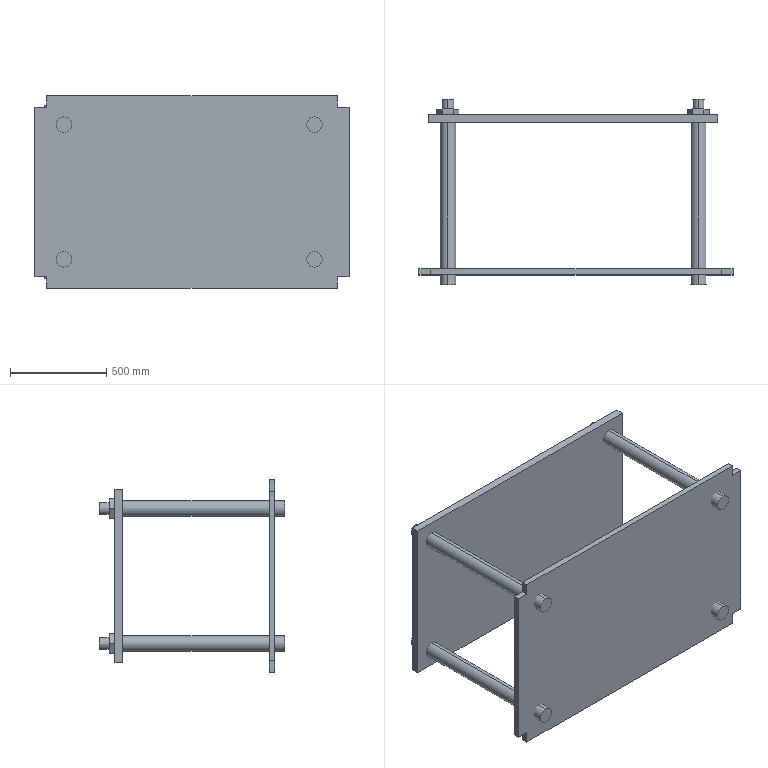Part | STEP file | PN_0018 Platform plate | 2 solids | 72 faces | box 1630 x 960 x 1000 mm | volume 120961919 mm3 | plane 56 | cylinder 16 | commonest cylinder face diameters 60 x8 80 x8